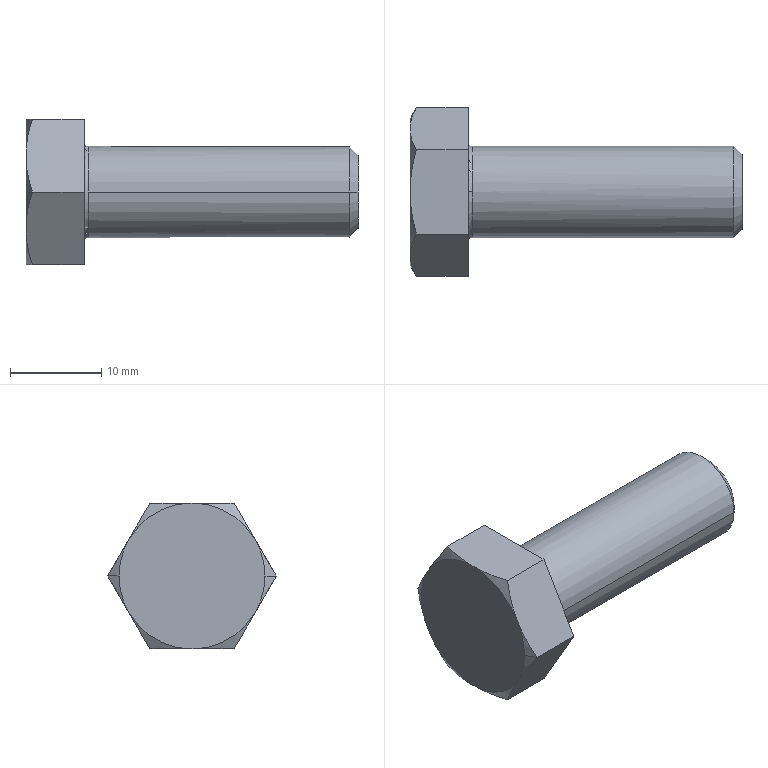Part | STEP file | KS B 1002 - C  M 10 x 30 | 1 solid | 23 faces | box 36.4 x 18.475 x 16 mm | volume 3759 mm3 | cone 10 | plane 9 | torus 2 | cylinder 2 | commonest cylinder face diameters 10 x2